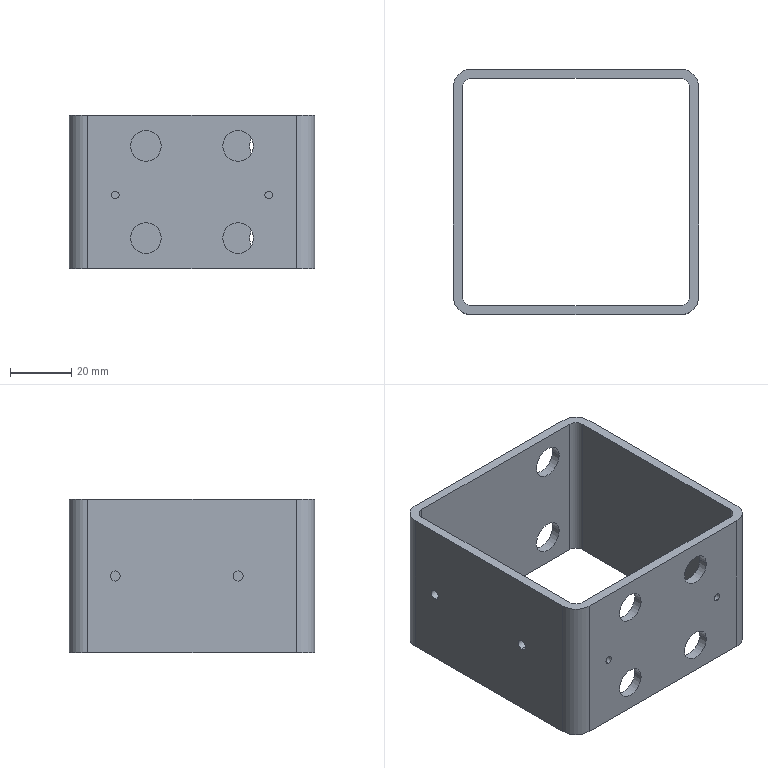Part | STEP file | X77-06302 | 1 solid | 38 faces | box 80 x 80 x 50 mm | volume 43498 mm3 | cylinder 28 | plane 10 | commonest cylinder face diameters 10 x8 2.5 x4 3.3 x4 6 x4 10.5 x4 12 x4
STEP:
#1=CARTESIAN_POINT('',(-19.91,-94.8,-15.));
#2=VERTEX_POINT('',#1);
#3=CARTESIAN_POINT('',(-29.91,-94.8,-15.));
#4=VERTEX_POINT('',#3);
#5=CARTESIAN_POINT('',(-24.91,-94.8,-15.));
#6=DIRECTION('',(0.,1.,0.));
#7=DIRECTION('',(0.,0.,-1.));
#8=AXIS2_PLACEMENT_3D('',#5,#6,#7);
#9=CIRCLE('',#8,5.);
#10=EDGE_CURVE('',#2,#4,#9,.T.);
#11=ORIENTED_EDGE('',*,*,#10,.T.);
#12=CARTESIAN_POINT('',(-29.91,-97.8,-15.));
#13=VERTEX_POINT('',#12);
#14=CARTESIAN_POINT('',(-29.91,-17.799,-15.));
#15=DIRECTION('',(0.,-1.,0.));
#16=VECTOR('',#15,1000.);
#17=LINE('',#14,#16);
#18=EDGE_CURVE('',#4,#13,#17,.T.);
#19=ORIENTED_EDGE('',*,*,#18,.T.);
#20=CARTESIAN_POINT('',(-19.91,-97.8,-15.));
#21=VERTEX_POINT('',#20);
#22=CARTESIAN_POINT('',(-24.91,-97.8,-15.));
#23=DIRECTION('',(0.,-1.,0.));
#24=DIRECTION('',(-1.,0.,0.));
#25=AXIS2_PLACEMENT_3D('',#22,#23,#24);
#26=CIRCLE('',#25,5.);
#27=EDGE_CURVE('',#13,#21,#26,.T.);
#28=ORIENTED_EDGE('',*,*,#27,.T.);
#29=CARTESIAN_POINT('',(-19.91,-17.799,-15.));
#30=DIRECTION('',(0.,-1.,0.));
#31=VECTOR('',#30,1000.);
#32=LINE('',#29,#31);
#33=EDGE_CURVE('',#2,#21,#32,.T.);
#34=ORIENTED_EDGE('',*,*,#33,.F.);
#35=EDGE_LOOP('',(#11,#19,#28,#34));
#36=FACE_OUTER_BOUND('',#35,.T.);
#37=CARTESIAN_POINT('',(-24.91,-17.799,-15.));
#38=DIRECTION('',(0.,-1.,0.));
#39=DIRECTION('',(1.,0.,0.));
#40=AXIS2_PLACEMENT_3D('',#37,#38,#39);
#41=CYLINDRICAL_SURFACE('',#40,5.);
#42=ADVANCED_FACE('',(#36),#41,.F.);
#43=CARTESIAN_POINT('',(10.09,-94.8,-15.));
#44=VERTEX_POINT('',#43);
#45=CARTESIAN_POINT('',(0.09,-94.8,-15.));
#46=VERTEX_POINT('',#45);
#47=CARTESIAN_POINT('',(5.09,-94.8,-15.));
#48=DIRECTION('',(0.,1.,0.));
#49=DIRECTION('',(0.,0.,-1.));
#50=AXIS2_PLACEMENT_3D('',#47,#48,#49);
#51=CIRCLE('',#50,5.);
#52=EDGE_CURVE('',#44,#46,#51,.T.);
#53=ORIENTED_EDGE('',*,*,#52,.T.);
#54=CARTESIAN_POINT('',(0.09,-97.8,-15.));
#55=VERTEX_POINT('',#54);
#56=CARTESIAN_POINT('',(0.09,-17.799,-15.));
#57=DIRECTION('',(0.,-1.,0.));
#58=VECTOR('',#57,1000.);
#59=LINE('',#56,#58);
#60=EDGE_CURVE('',#46,#55,#59,.T.);
#61=ORIENTED_EDGE('',*,*,#60,.T.);
#62=CARTESIAN_POINT('',(10.09,-97.8,-15.));
#63=VERTEX_POINT('',#62);
#64=CARTESIAN_POINT('',(5.09,-97.8,-15.));
#65=DIRECTION('',(0.,-1.,0.));
#66=DIRECTION('',(-1.,0.,0.));
#67=AXIS2_PLACEMENT_3D('',#64,#65,#66);
#68=CIRCLE('',#67,5.);
#69=EDGE_CURVE('',#55,#63,#68,.T.);
#70=ORIENTED_EDGE('',*,*,#69,.T.);
#71=CARTESIAN_POINT('',(10.09,-17.799,-15.));
#72=DIRECTION('',(0.,-1.,0.));
#73=VECTOR('',#72,1000.);
#74=LINE('',#71,#73);
#75=EDGE_CURVE('',#44,#63,#74,.T.);
#76=ORIENTED_EDGE('',*,*,#75,.F.);
#77=EDGE_LOOP('',(#53,#61,#70,#76));
#78=FACE_OUTER_BOUND('',#77,.T.);
#79=CARTESIAN_POINT('',(5.09,-17.799,-15.));
#80=DIRECTION('',(0.,-1.,0.));
#81=DIRECTION('',(1.,0.,0.));
#82=AXIS2_PLACEMENT_3D('',#79,#80,#81);
#83=CYLINDRICAL_SURFACE('',#82,5.);
#84=ADVANCED_FACE('',(#78),#83,.F.);
#85=CARTESIAN_POINT('',(-19.91,-94.8,15.));
#86=VERTEX_POINT('',#85);
#87=CARTESIAN_POINT('',(-29.91,-94.8,15.));
#88=VERTEX_POINT('',#87);
#89=CARTESIAN_POINT('',(-24.91,-94.8,15.));
#90=DIRECTION('',(0.,1.,0.));
#91=DIRECTION('',(0.,0.,-1.));
#92=AXIS2_PLACEMENT_3D('',#89,#90,#91);
#93=CIRCLE('',#92,5.);
#94=EDGE_CURVE('',#86,#88,#93,.T.);
#95=ORIENTED_EDGE('',*,*,#94,.T.);
#96=CARTESIAN_POINT('',(-29.91,-97.8,15.));
#97=VERTEX_POINT('',#96);
#98=CARTESIAN_POINT('',(-29.91,-17.799,15.));
#99=DIRECTION('',(0.,-1.,0.));
#100=VECTOR('',#99,1000.);
#101=LINE('',#98,#100);
#102=EDGE_CURVE('',#88,#97,#101,.T.);
#103=ORIENTED_EDGE('',*,*,#102,.T.);
#104=CARTESIAN_POINT('',(-19.91,-97.8,15.));
#105=VERTEX_POINT('',#104);
#106=CARTESIAN_POINT('',(-24.91,-97.8,15.));
#107=DIRECTION('',(0.,-1.,0.));
#108=DIRECTION('',(1.,0.,0.));
#109=AXIS2_PLACEMENT_3D('',#106,#107,#108);
#110=CIRCLE('',#109,5.);
#111=EDGE_CURVE('',#97,#105,#110,.T.);
#112=ORIENTED_EDGE('',*,*,#111,.T.);
#113=CARTESIAN_POINT('',(-19.91,-17.799,15.));
#114=DIRECTION('',(0.,-1.,0.));
#115=VECTOR('',#114,1000.);
#116=LINE('',#113,#115);
#117=EDGE_CURVE('',#86,#105,#116,.T.);
#118=ORIENTED_EDGE('',*,*,#117,.F.);
#119=EDGE_LOOP('',(#95,#103,#112,#118));
#120=FACE_OUTER_BOUND('',#119,.T.);
#121=CARTESIAN_POINT('',(-24.91,-17.799,15.));
#122=DIRECTION('',(0.,-1.,0.));
#123=DIRECTION('',(1.,0.,0.));
#124=AXIS2_PLACEMENT_3D('',#121,#122,#123);
#125=CYLINDRICAL_SURFACE('',#124,5.);
#126=ADVANCED_FACE('',(#120),#125,.F.);
#127=CARTESIAN_POINT('',(10.09,-94.8,15.));
#128=VERTEX_POINT('',#127);
#129=CARTESIAN_POINT('',(0.09,-94.8,15.));
#130=VERTEX_POINT('',#129);
#131=CARTESIAN_POINT('',(5.09,-94.8,15.));
#132=DIRECTION('',(0.,1.,0.));
#133=DIRECTION('',(0.,0.,-1.));
#134=AXIS2_PLACEMENT_3D('',#131,#132,#133);
#135=CIRCLE('',#134,5.);
#136=EDGE_CURVE('',#128,#130,#135,.T.);
#137=ORIENTED_EDGE('',*,*,#136,.T.);
#138=CARTESIAN_POINT('',(0.09,-97.8,15.));
#139=VERTEX_POINT('',#138);
#140=CARTESIAN_POINT('',(0.09,-17.799,15.));
#141=DIRECTION('',(0.,-1.,0.));
#142=VECTOR('',#141,1000.);
#143=LINE('',#140,#142);
#144=EDGE_CURVE('',#130,#139,#143,.T.);
#145=ORIENTED_EDGE('',*,*,#144,.T.);
#146=CARTESIAN_POINT('',(10.09,-97.8,15.));
#147=VERTEX_POINT('',#146);
#148=CARTESIAN_POINT('',(5.09,-97.8,15.));
#149=DIRECTION('',(0.,-1.,0.));
#150=DIRECTION('',(1.,0.,0.));
#151=AXIS2_PLACEMENT_3D('',#148,#149,#150);
#152=CIRCLE('',#151,5.);
#153=EDGE_CURVE('',#139,#147,#152,.T.);
#154=ORIENTED_EDGE('',*,*,#153,.T.);
#155=CARTESIAN_POINT('',(10.09,-17.799,15.));
#156=DIRECTION('',(0.,-1.,0.));
#157=VECTOR('',#156,1000.);
#158=LINE('',#155,#157);
#159=EDGE_CURVE('',#128,#147,#158,.T.);
#160=ORIENTED_EDGE('',*,*,#159,.F.);
#161=EDGE_LOOP('',(#137,#145,#154,#160));
#162=FACE_OUTER_BOUND('',#161,.T.);
#163=CARTESIAN_POINT('',(5.09,-17.799,15.));
#164=DIRECTION('',(0.,-1.,0.));
#165=DIRECTION('',(1.,0.,0.));
#166=AXIS2_PLACEMENT_3D('',#163,#164,#165);
#167=CYLINDRICAL_SURFACE('',#166,5.);
#168=ADVANCED_FACE('',(#162),#167,.F.);
#169=CARTESIAN_POINT('',(-34.91,-94.8,0.25));
#170=VERTEX_POINT('',#169);
#171=CARTESIAN_POINT('',(-34.91,-94.8,-2.25));
#172=VERTEX_POINT('',#171);
#173=CARTESIAN_POINT('',(-34.91,-94.8,-1.));
#174=DIRECTION('',(0.,-1.,0.));
#175=DIRECTION('',(0.,0.,-1.));
#176=AXIS2_PLACEMENT_3D('',#173,#174,#175);
#177=CIRCLE('',#176,1.25);
#178=EDGE_CURVE('',#170,#172,#177,.T.);
#179=ORIENTED_EDGE('',*,*,#178,.F.);
#180=CARTESIAN_POINT('',(-34.91,-97.8,0.25));
#181=VERTEX_POINT('',#180);
#182=CARTESIAN_POINT('',(-34.91,-97.8,0.25));
#183=DIRECTION('',(0.,-1.,0.));
#184=VECTOR('',#183,1000.);
#185=LINE('',#182,#184);
#186=EDGE_CURVE('',#170,#181,#185,.T.);
#187=ORIENTED_EDGE('',*,*,#186,.T.);
#188=CARTESIAN_POINT('',(-34.91,-97.8,-2.25));
#189=VERTEX_POINT('',#188);
#190=CARTESIAN_POINT('',(-34.91,-97.8,-1.));
#191=DIRECTION('',(0.,-1.,0.));
#192=DIRECTION('',(0.,0.,-1.));
#193=AXIS2_PLACEMENT_3D('',#190,#191,#192);
#194=CIRCLE('',#193,1.25);
#195=EDGE_CURVE('',#181,#189,#194,.T.);
#196=ORIENTED_EDGE('',*,*,#195,.T.);
#197=CARTESIAN_POINT('',(-34.91,-97.8,-2.25));
#198=DIRECTION('',(0.,-1.,0.));
#199=VECTOR('',#198,1000.);
#200=LINE('',#197,#199);
#201=EDGE_CURVE('',#172,#189,#200,.T.);
#202=ORIENTED_EDGE('',*,*,#201,.F.);
#203=EDGE_LOOP('',(#179,#187,#196,#202));
#204=FACE_OUTER_BOUND('',#203,.T.);
#205=CARTESIAN_POINT('',(-34.91,-97.8,-1.));
#206=DIRECTION('',(0.,-1.,0.));
#207=DIRECTION('',(0.,0.,-1.));
#208=AXIS2_PLACEMENT_3D('',#205,#206,#207);
#209=CYLINDRICAL_SURFACE('',#208,1.25);
#210=ADVANCED_FACE('',(#204),#209,.F.);
#211=CARTESIAN_POINT('',(15.09,-94.8,0.25));
#212=VERTEX_POINT('',#211);
#213=CARTESIAN_POINT('',(15.09,-94.8,-2.25));
#214=VERTEX_POINT('',#213);
#215=CARTESIAN_POINT('',(15.09,-94.8,-1.));
#216=DIRECTION('',(0.,-1.,0.));
#217=DIRECTION('',(0.,0.,-1.));
#218=AXIS2_PLACEMENT_3D('',#215,#216,#217);
#219=CIRCLE('',#218,1.25);
#220=EDGE_CURVE('',#212,#214,#219,.T.);
#221=ORIENTED_EDGE('',*,*,#220,.F.);
#222=CARTESIAN_POINT('',(15.09,-97.8,0.25));
#223=VERTEX_POINT('',#222);
#224=CARTESIAN_POINT('',(15.09,-97.8,0.25));
#225=DIRECTION('',(0.,-1.,0.));
#226=VECTOR('',#225,1000.);
#227=LINE('',#224,#226);
#228=EDGE_CURVE('',#212,#223,#227,.T.);
#229=ORIENTED_EDGE('',*,*,#228,.T.);
#230=CARTESIAN_POINT('',(15.09,-97.8,-2.25));
#231=VERTEX_POINT('',#230);
#232=CARTESIAN_POINT('',(15.09,-97.8,-1.));
#233=DIRECTION('',(0.,-1.,0.));
#234=DIRECTION('',(0.,0.,-1.));
#235=AXIS2_PLACEMENT_3D('',#232,#233,#234);
#236=CIRCLE('',#235,1.25);
#237=EDGE_CURVE('',#223,#231,#236,.T.);
#238=ORIENTED_EDGE('',*,*,#237,.T.);
#239=CARTESIAN_POINT('',(15.09,-97.8,-2.25));
#240=DIRECTION('',(0.,-1.,0.));
#241=VECTOR('',#240,1000.);
#242=LINE('',#239,#241);
#243=EDGE_CURVE('',#214,#231,#242,.T.);
#244=ORIENTED_EDGE('',*,*,#243,.F.);
#245=EDGE_LOOP('',(#221,#229,#238,#244));
#246=FACE_OUTER_BOUND('',#245,.T.);
#247=CARTESIAN_POINT('',(15.09,-97.8,-1.));
#248=DIRECTION('',(0.,-1.,0.));
#249=DIRECTION('',(0.,0.,-1.));
#250=AXIS2_PLACEMENT_3D('',#247,#248,#249);
#251=CYLINDRICAL_SURFACE('',#250,1.25);
#252=ADVANCED_FACE('',(#246),#251,.F.);
#253=CARTESIAN_POINT('',(8.84,-17.8,-15.));
#254=VERTEX_POINT('',#253);
#255=CARTESIAN_POINT('',(19.34,-17.8,-15.));
#256=VERTEX_POINT('',#255);
#257=CARTESIAN_POINT('',(14.09,-17.8,-15.));
#258=DIRECTION('',(0.,-1.,0.));
#259=DIRECTION('',(1.,0.,0.));
#260=AXIS2_PLACEMENT_3D('',#257,#258,#259);
#261=CIRCLE('',#260,5.25);
#262=EDGE_CURVE('',#254,#256,#261,.T.);
#263=ORIENTED_EDGE('',*,*,#262,.F.);
#264=CARTESIAN_POINT('',(8.84,-20.8,-15.));
#265=VERTEX_POINT('',#264);
#266=CARTESIAN_POINT('',(8.84,-17.8,-15.));
#267=DIRECTION('',(0.,-1.,0.));
#268=VECTOR('',#267,1000.);
#269=LINE('',#266,#268);
#270=EDGE_CURVE('',#254,#265,#269,.T.);
#271=ORIENTED_EDGE('',*,*,#270,.T.);
#272=CARTESIAN_POINT('',(19.34,-20.8,-15.));
#273=VERTEX_POINT('',#272);
#274=CARTESIAN_POINT('',(14.09,-20.8,-15.));
#275=DIRECTION('',(0.,-1.,0.));
#276=DIRECTION('',(1.,0.,0.));
#277=AXIS2_PLACEMENT_3D('',#274,#275,#276);
#278=CIRCLE('',#277,5.25);
#279=EDGE_CURVE('',#265,#273,#278,.T.);
#280=ORIENTED_EDGE('',*,*,#279,.T.);
#281=CARTESIAN_POINT('',(19.34,-17.8,-15.));
#282=DIRECTION('',(0.,-1.,0.));
#283=VECTOR('',#282,1000.);
#284=LINE('',#281,#283);
#285=EDGE_CURVE('',#256,#273,#284,.T.);
#286=ORIENTED_EDGE('',*,*,#285,.F.);
#287=EDGE_LOOP('',(#263,#271,#280,#286));
#288=FACE_OUTER_BOUND('',#287,.T.);
#289=CARTESIAN_POINT('',(14.09,-17.8,-15.));
#290=DIRECTION('',(0.,-1.,0.));
#291=DIRECTION('',(1.,0.,0.));
#292=AXIS2_PLACEMENT_3D('',#289,#290,#291);
#293=CYLINDRICAL_SURFACE('',#292,5.25);
#294=ADVANCED_FACE('',(#288),#293,.F.);
#295=CARTESIAN_POINT('',(8.84,-17.8,15.));
#296=VERTEX_POINT('',#295);
#297=CARTESIAN_POINT('',(19.34,-17.8,15.));
#298=VERTEX_POINT('',#297);
#299=CARTESIAN_POINT('',(14.09,-17.8,15.));
#300=DIRECTION('',(0.,-1.,0.));
#301=DIRECTION('',(1.,0.,0.));
#302=AXIS2_PLACEMENT_3D('',#299,#300,#301);
#303=CIRCLE('',#302,5.25);
#304=EDGE_CURVE('',#296,#298,#303,.T.);
#305=ORIENTED_EDGE('',*,*,#304,.F.);
#306=CARTESIAN_POINT('',(8.84,-20.8,15.));
#307=VERTEX_POINT('',#306);
#308=CARTESIAN_POINT('',(8.84,-17.8,15.));
#309=DIRECTION('',(0.,-1.,0.));
#310=VECTOR('',#309,1000.);
#311=LINE('',#308,#310);
#312=EDGE_CURVE('',#296,#307,#311,.T.);
#313=ORIENTED_EDGE('',*,*,#312,.T.);
#314=CARTESIAN_POINT('',(19.34,-20.8,15.));
#315=VERTEX_POINT('',#314);
#316=CARTESIAN_POINT('',(14.09,-20.8,15.));
#317=DIRECTION('',(0.,-1.,0.));
#318=DIRECTION('',(1.,0.,0.));
#319=AXIS2_PLACEMENT_3D('',#316,#317,#318);
#320=CIRCLE('',#319,5.25);
#321=EDGE_CURVE('',#307,#315,#320,.T.);
#322=ORIENTED_EDGE('',*,*,#321,.T.);
#323=CARTESIAN_POINT('',(19.34,-17.8,15.));
#324=DIRECTION('',(0.,-1.,0.));
#325=VECTOR('',#324,1000.);
#326=LINE('',#323,#325);
#327=EDGE_CURVE('',#298,#315,#326,.T.);
#328=ORIENTED_EDGE('',*,*,#327,.F.);
#329=EDGE_LOOP('',(#305,#313,#322,#328));
#330=FACE_OUTER_BOUND('',#329,.T.);
#331=CARTESIAN_POINT('',(14.09,-17.8,15.));
#332=DIRECTION('',(0.,-1.,0.));
#333=DIRECTION('',(1.,0.,0.));
#334=AXIS2_PLACEMENT_3D('',#331,#332,#333);
#335=CYLINDRICAL_SURFACE('',#334,5.25);
#336=ADVANCED_FACE('',(#330),#335,.F.);
#337=CARTESIAN_POINT('',(-46.91,-72.8,-1.65));
#338=VERTEX_POINT('',#337);
#339=CARTESIAN_POINT('',(-46.91,-72.8,1.65));
#340=VERTEX_POINT('',#339);
#341=CARTESIAN_POINT('',(-46.91,-72.8,0.));
#342=DIRECTION('',(-1.,0.,0.));
#343=DIRECTION('',(0.,-1.,0.));
#344=AXIS2_PLACEMENT_3D('',#341,#342,#343);
#345=CIRCLE('',#344,1.65);
#346=EDGE_CURVE('',#338,#340,#345,.T.);
#347=ORIENTED_EDGE('',*,*,#346,.F.);
#348=CARTESIAN_POINT('',(-49.91,-72.8,-1.65));
#349=VERTEX_POINT('',#348);
#350=CARTESIAN_POINT('',(-49.91,-72.8,-1.65));
#351=DIRECTION('',(-1.,0.,0.));
#352=VECTOR('',#351,1000.);
#353=LINE('',#350,#352);
#354=EDGE_CURVE('',#338,#349,#353,.T.);
#355=ORIENTED_EDGE('',*,*,#354,.T.);
#356=CARTESIAN_POINT('',(-49.91,-72.8,1.65));
#357=VERTEX_POINT('',#356);
#358=CARTESIAN_POINT('',(-49.91,-72.8,0.));
#359=DIRECTION('',(-1.,0.,0.));
#360=DIRECTION('',(0.,0.,1.));
#361=AXIS2_PLACEMENT_3D('',#358,#359,#360);
#362=CIRCLE('',#361,1.65);
#363=EDGE_CURVE('',#349,#357,#362,.T.);
#364=ORIENTED_EDGE('',*,*,#363,.T.);
#365=CARTESIAN_POINT('',(-49.91,-72.8,1.65));
#366=DIRECTION('',(-1.,0.,0.));
#367=VECTOR('',#366,1000.);
#368=LINE('',#365,#367);
#369=EDGE_CURVE('',#340,#357,#368,.T.);
#370=ORIENTED_EDGE('',*,*,#369,.F.);
#371=EDGE_LOOP('',(#347,#355,#364,#370));
#372=FACE_OUTER_BOUND('',#371,.T.);
#373=CARTESIAN_POINT('',(-49.91,-72.8,0.));
#374=DIRECTION('',(-1.,0.,0.));
#375=DIRECTION('',(0.,0.,1.));
#376=AXIS2_PLACEMENT_3D('',#373,#374,#375);
#377=CYLINDRICAL_SURFACE('',#376,1.65);
#378=ADVANCED_FACE('',(#372),#377,.F.);
#379=CARTESIAN_POINT('',(-46.91,-32.8,-1.65));
#380=VERTEX_POINT('',#379);
#381=CARTESIAN_POINT('',(-46.91,-32.8,1.65));
#382=VERTEX_POINT('',#381);
#383=CARTESIAN_POINT('',(-46.91,-32.8,0.));
#384=DIRECTION('',(-1.,0.,0.));
#385=DIRECTION('',(0.,-1.,0.));
#386=AXIS2_PLACEMENT_3D('',#383,#384,#385);
#387=CIRCLE('',#386,1.65);
#388=EDGE_CURVE('',#380,#382,#387,.T.);
#389=ORIENTED_EDGE('',*,*,#388,.F.);
#390=CARTESIAN_POINT('',(-49.91,-32.8,-1.65));
#391=VERTEX_POINT('',#390);
#392=CARTESIAN_POINT('',(-49.91,-32.8,-1.65));
#393=DIRECTION('',(-1.,0.,0.));
#394=VECTOR('',#393,1000.);
#395=LINE('',#392,#394);
#396=EDGE_CURVE('',#380,#391,#395,.T.);
#397=ORIENTED_EDGE('',*,*,#396,.T.);
#398=CARTESIAN_POINT('',(-49.91,-32.8,1.65));
#399=VERTEX_POINT('',#398);
#400=CARTESIAN_POINT('',(-49.91,-32.8,0.));
#401=DIRECTION('',(-1.,0.,0.));
#402=DIRECTION('',(0.,0.,1.));
#403=AXIS2_PLACEMENT_3D('',#400,#401,#402);
#404=CIRCLE('',#403,1.65);
#405=EDGE_CURVE('',#391,#399,#404,.T.);
#406=ORIENTED_EDGE('',*,*,#405,.T.);
#407=CARTESIAN_POINT('',(-49.91,-32.8,1.65));
#408=DIRECTION('',(-1.,0.,0.));
#409=VECTOR('',#408,1000.);
#410=LINE('',#407,#409);
#411=EDGE_CURVE('',#382,#399,#410,.T.);
#412=ORIENTED_EDGE('',*,*,#411,.F.);
#413=EDGE_LOOP('',(#389,#397,#406,#412));
#414=FACE_OUTER_BOUND('',#413,.T.);
#415=CARTESIAN_POINT('',(-49.91,-32.8,0.));
#416=DIRECTION('',(-1.,0.,0.));
#417=DIRECTION('',(0.,0.,1.));
#418=AXIS2_PLACEMENT_3D('',#415,#416,#417);
#419=CYLINDRICAL_SURFACE('',#418,1.65);
#420=ADVANCED_FACE('',(#414),#419,.F.);
#421=CARTESIAN_POINT('',(-49.91,-23.8,-25.));
#422=VERTEX_POINT('',#421);
#423=CARTESIAN_POINT('',(-49.91,-23.8,25.));
#424=VERTEX_POINT('',#423);
#425=CARTESIAN_POINT('',(-49.91,-23.8,-25.));
#426=DIRECTION('',(0.,0.,1.));
#427=VECTOR('',#426,1000.);
#428=LINE('',#425,#427);
#429=EDGE_CURVE('',#422,#424,#428,.T.);
#430=ORIENTED_EDGE('',*,*,#429,.T.);
#431=CARTESIAN_POINT('',(-43.91,-17.8,25.));
#432=VERTEX_POINT('',#431);
#433=CARTESIAN_POINT('',(-43.91,-23.8,25.));
#434=DIRECTION('',(0.,0.,1.));
#435=DIRECTION('',(-1.,0.,0.));
#436=AXIS2_PLACEMENT_3D('',#433,#434,#435);
#437=CIRCLE('',#436,6.);
#438=EDGE_CURVE('',#432,#424,#437,.T.);
#439=ORIENTED_EDGE('',*,*,#438,.F.);
#440=CARTESIAN_POINT('',(-43.91,-17.8,-25.));
#441=VERTEX_POINT('',#440);
#442=CARTESIAN_POINT('',(-43.91,-17.8,-25.));
#443=DIRECTION('',(0.,0.,1.));
#444=VECTOR('',#443,1000.);
#445=LINE('',#442,#444);
#446=EDGE_CURVE('',#441,#432,#445,.T.);
#447=ORIENTED_EDGE('',*,*,#446,.F.);
#448=CARTESIAN_POINT('',(-43.91,-23.8,-25.));
#449=DIRECTION('',(0.,0.,1.));
#450=DIRECTION('',(-1.,0.,0.));
#451=AXIS2_PLACEMENT_3D('',#448,#449,#450);
#452=CIRCLE('',#451,6.);
#453=EDGE_CURVE('',#441,#422,#452,.T.);
#454=ORIENTED_EDGE('',*,*,#453,.T.);
#455=EDGE_LOOP('',(#430,#439,#447,#454));
#456=FACE_OUTER_BOUND('',#455,.T.);
#457=CARTESIAN_POINT('',(-43.91,-23.8,-25.));
#458=DIRECTION('',(0.,0.,1.));
#459=DIRECTION('',(1.,0.,0.));
#460=AXIS2_PLACEMENT_3D('',#457,#458,#459);
#461=CYLINDRICAL_SURFACE('',#460,6.);
#462=ADVANCED_FACE('',(#456),#461,.T.);
#463=CARTESIAN_POINT('',(14.09,-17.8,-15.));
#464=DIRECTION('',(0.,-1.,0.));
#465=DIRECTION('',(1.,0.,0.));
#466=AXIS2_PLACEMENT_3D('',#463,#464,#465);
#467=CIRCLE('',#466,5.25);
#468=EDGE_CURVE('',#256,#254,#467,.T.);
#469=ORIENTED_EDGE('',*,*,#468,.T.);
#470=ORIENTED_EDGE('',*,*,#262,.T.);
#471=EDGE_LOOP('',(#469,#470));
#472=FACE_BOUND('',#471,.T.);
#473=CARTESIAN_POINT('',(14.09,-17.8,15.));
#474=DIRECTION('',(0.,-1.,0.));
#475=DIRECTION('',(1.,0.,0.));
#476=AXIS2_PLACEMENT_3D('',#473,#474,#475);
#477=CIRCLE('',#476,5.25);
#478=EDGE_CURVE('',#298,#296,#477,.T.);
#479=ORIENTED_EDGE('',*,*,#478,.T.);
#480=ORIENTED_EDGE('',*,*,#304,.T.);
#481=EDGE_LOOP('',(#479,#480));
#482=FACE_BOUND('',#481,.T.);
#483=ORIENTED_EDGE('',*,*,#446,.T.);
#484=CARTESIAN_POINT('',(24.09,-17.8,25.));
#485=VERTEX_POINT('',#484);
#486=CARTESIAN_POINT('',(24.09,-17.8,25.));
#487=DIRECTION('',(-1.,0.,0.));
#488=VECTOR('',#487,1000.);
#489=LINE('',#486,#488);
#490=EDGE_CURVE('',#485,#432,#489,.T.);
#491=ORIENTED_EDGE('',*,*,#490,.F.);
#492=CARTESIAN_POINT('',(24.09,-17.8,-25.));
#493=VERTEX_POINT('',#492);
#494=CARTESIAN_POINT('',(24.09,-17.8,-25.));
#495=DIRECTION('',(0.,0.,1.));
#496=VECTOR('',#495,1000.);
#497=LINE('',#494,#496);
#498=EDGE_CURVE('',#493,#485,#497,.T.);
#499=ORIENTED_EDGE('',*,*,#498,.F.);
#500=CARTESIAN_POINT('',(24.09,-17.8,-25.));
#501=DIRECTION('',(-1.,0.,0.));
#502=VECTOR('',#501,1000.);
#503=LINE('',#500,#502);
#504=EDGE_CURVE('',#493,#441,#503,.T.);
#505=ORIENTED_EDGE('',*,*,#504,.T.);
#506=EDGE_LOOP('',(#483,#491,#499,#505));
#507=FACE_OUTER_BOUND('',#506,.T.);
#508=CARTESIAN_POINT('',(24.09,-17.8,-25.));
#509=DIRECTION('',(0.,1.,0.));
#510=DIRECTION('',(-1.,0.,0.));
#511=AXIS2_PLACEMENT_3D('',#508,#509,#510);
#512=PLANE('',#511);
#513=ADVANCED_FACE('',(#472,#482,#507),#512,.T.);
#514=ORIENTED_EDGE('',*,*,#498,.T.);
#515=CARTESIAN_POINT('',(30.09,-23.8,25.));
#516=VERTEX_POINT('',#515);
#517=CARTESIAN_POINT('',(24.09,-23.8,25.));
#518=DIRECTION('',(0.,0.,1.));
#519=DIRECTION('',(1.,0.,0.));
#520=AXIS2_PLACEMENT_3D('',#517,#518,#519);
#521=CIRCLE('',#520,6.);
#522=EDGE_CURVE('',#516,#485,#521,.T.);
#523=ORIENTED_EDGE('',*,*,#522,.F.);
#524=CARTESIAN_POINT('',(30.09,-23.8,-25.));
#525=VERTEX_POINT('',#524);
#526=CARTESIAN_POINT('',(30.09,-23.8,-25.));
#527=DIRECTION('',(0.,0.,1.));
#528=VECTOR('',#527,1000.);
#529=LINE('',#526,#528);
#530=EDGE_CURVE('',#525,#516,#529,.T.);
#531=ORIENTED_EDGE('',*,*,#530,.F.);
#532=CARTESIAN_POINT('',(24.09,-23.8,-25.));
#533=DIRECTION('',(0.,0.,1.));
#534=DIRECTION('',(1.,0.,0.));
#535=AXIS2_PLACEMENT_3D('',#532,#533,#534);
#536=CIRCLE('',#535,6.);
#537=EDGE_CURVE('',#525,#493,#536,.T.);
#538=ORIENTED_EDGE('',*,*,#537,.T.);
#539=EDGE_LOOP('',(#514,#523,#531,#538));
#540=FACE_OUTER_BOUND('',#539,.T.);
#541=CARTESIAN_POINT('',(24.09,-23.8,-25.));
#542=DIRECTION('',(0.,0.,1.));
#543=DIRECTION('',(1.,0.,0.));
#544=AXIS2_PLACEMENT_3D('',#541,#542,#543);
#545=CYLINDRICAL_SURFACE('',#544,6.);
#546=ADVANCED_FACE('',(#540),#545,.T.);
#547=ORIENTED_EDGE('',*,*,#530,.T.);
#548=CARTESIAN_POINT('',(30.09,-91.8,25.));
#549=VERTEX_POINT('',#548);
#550=CARTESIAN_POINT('',(30.09,-23.8,25.));
#551=DIRECTION('',(0.,1.,0.));
#552=VECTOR('',#551,1000.);
#553=LINE('',#550,#552);
#554=EDGE_CURVE('',#549,#516,#553,.T.);
#555=ORIENTED_EDGE('',*,*,#554,.F.);
#556=CARTESIAN_POINT('',(30.09,-91.8,-25.));
#557=VERTEX_POINT('',#556);
#558=CARTESIAN_POINT('',(30.09,-91.8,-25.));
#559=DIRECTION('',(0.,0.,1.));
#560=VECTOR('',#559,1000.);
#561=LINE('',#558,#560);
#562=EDGE_CURVE('',#557,#549,#561,.T.);
#563=ORIENTED_EDGE('',*,*,#562,.F.);
#564=CARTESIAN_POINT('',(30.09,-23.8,-25.));
#565=DIRECTION('',(0.,1.,0.));
#566=VECTOR('',#565,1000.);
#567=LINE('',#564,#566);
#568=EDGE_CURVE('',#557,#525,#567,.T.);
#569=ORIENTED_EDGE('',*,*,#568,.T.);
#570=EDGE_LOOP('',(#547,#555,#563,#569));
#571=FACE_OUTER_BOUND('',#570,.T.);
#572=CARTESIAN_POINT('',(30.09,-23.8,-25.));
#573=DIRECTION('',(1.,0.,0.));
#574=DIRECTION('',(0.,1.,0.));
#575=AXIS2_PLACEMENT_3D('',#572,#573,#574);
#576=PLANE('',#575);
#577=ADVANCED_FACE('',(#571),#576,.T.);
#578=ORIENTED_EDGE('',*,*,#562,.T.);
#579=CARTESIAN_POINT('',(24.09,-97.8,25.));
#580=VERTEX_POINT('',#579);
#581=CARTESIAN_POINT('',(24.09,-91.8,25.));
#582=DIRECTION('',(0.,0.,1.));
#583=DIRECTION('',(-1.,0.,0.));
#584=AXIS2_PLACEMENT_3D('',#581,#582,#583);
#585=CIRCLE('',#584,6.);
#586=EDGE_CURVE('',#580,#549,#585,.T.);
#587=ORIENTED_EDGE('',*,*,#586,.F.);
#588=CARTESIAN_POINT('',(24.09,-97.8,-25.));
#589=VERTEX_POINT('',#588);
#590=CARTESIAN_POINT('',(24.09,-97.8,-25.));
#591=DIRECTION('',(0.,0.,1.));
#592=VECTOR('',#591,1000.);
#593=LINE('',#590,#592);
#594=EDGE_CURVE('',#589,#580,#593,.T.);
#595=ORIENTED_EDGE('',*,*,#594,.F.);
#596=CARTESIAN_POINT('',(24.09,-91.8,-25.));
#597=DIRECTION('',(0.,0.,1.));
#598=DIRECTION('',(-1.,0.,0.));
#599=AXIS2_PLACEMENT_3D('',#596,#597,#598);
#600=CIRCLE('',#599,6.);
#601=EDGE_CURVE('',#589,#557,#600,.T.);
#602=ORIENTED_EDGE('',*,*,#601,.T.);
#603=EDGE_LOOP('',(#578,#587,#595,#602));
#604=FACE_OUTER_BOUND('',#603,.T.);
#605=CARTESIAN_POINT('',(24.09,-91.8,-25.));
#606=DIRECTION('',(0.,0.,1.));
#607=DIRECTION('',(1.,0.,0.));
#608=AXIS2_PLACEMENT_3D('',#605,#606,#607);
#609=CYLINDRICAL_SURFACE('',#608,6.);
#610=ADVANCED_FACE('',(#604),#609,.T.);
#611=CARTESIAN_POINT('',(-24.91,-97.8,-15.));
#612=DIRECTION('',(0.,-1.,0.));
#613=DIRECTION('',(-1.,0.,0.));
#614=AXIS2_PLACEMENT_3D('',#611,#612,#613);
#615=CIRCLE('',#614,5.);
#616=EDGE_CURVE('',#21,#13,#615,.T.);
#617=ORIENTED_EDGE('',*,*,#616,.F.);
#618=ORIENTED_EDGE('',*,*,#27,.F.);
#619=EDGE_LOOP('',(#617,#618));
#620=FACE_BOUND('',#619,.T.);
#621=CARTESIAN_POINT('',(5.09,-97.8,-15.));
#622=DIRECTION('',(0.,-1.,0.));
#623=DIRECTION('',(-1.,0.,0.));
#624=AXIS2_PLACEMENT_3D('',#621,#622,#623);
#625=CIRCLE('',#624,5.);
#626=EDGE_CURVE('',#63,#55,#625,.T.);
#627=ORIENTED_EDGE('',*,*,#626,.F.);
#628=ORIENTED_EDGE('',*,*,#69,.F.);
#629=EDGE_LOOP('',(#627,#628));
#630=FACE_BOUND('',#629,.T.);
#631=CARTESIAN_POINT('',(-24.91,-97.8,15.));
#632=DIRECTION('',(0.,-1.,0.));
#633=DIRECTION('',(1.,0.,0.));
#634=AXIS2_PLACEMENT_3D('',#631,#632,#633);
#635=CIRCLE('',#634,5.);
#636=EDGE_CURVE('',#105,#97,#635,.T.);
#637=ORIENTED_EDGE('',*,*,#636,.F.);
#638=ORIENTED_EDGE('',*,*,#111,.F.);
#639=EDGE_LOOP('',(#637,#638));
#640=FACE_BOUND('',#639,.T.);
#641=CARTESIAN_POINT('',(5.09,-97.8,15.));
#642=DIRECTION('',(0.,-1.,0.));
#643=DIRECTION('',(1.,0.,0.));
#644=AXIS2_PLACEMENT_3D('',#641,#642,#643);
#645=CIRCLE('',#644,5.);
#646=EDGE_CURVE('',#147,#139,#645,.T.);
#647=ORIENTED_EDGE('',*,*,#646,.F.);
#648=ORIENTED_EDGE('',*,*,#153,.F.);
#649=EDGE_LOOP('',(#647,#648));
#650=FACE_BOUND('',#649,.T.);
#651=CARTESIAN_POINT('',(-34.91,-97.8,-1.));
#652=DIRECTION('',(0.,-1.,0.));
#653=DIRECTION('',(0.,0.,-1.));
#654=AXIS2_PLACEMENT_3D('',#651,#652,#653);
#655=CIRCLE('',#654,1.25);
#656=EDGE_CURVE('',#189,#181,#655,.T.);
#657=ORIENTED_EDGE('',*,*,#656,.F.);
#658=ORIENTED_EDGE('',*,*,#195,.F.);
#659=EDGE_LOOP('',(#657,#658));
#660=FACE_BOUND('',#659,.T.);
#661=CARTESIAN_POINT('',(15.09,-97.8,-1.));
#662=DIRECTION('',(0.,-1.,0.));
#663=DIRECTION('',(0.,0.,-1.));
#664=AXIS2_PLACEMENT_3D('',#661,#662,#663);
#665=CIRCLE('',#664,1.25);
#666=EDGE_CURVE('',#231,#223,#665,.T.);
#667=ORIENTED_EDGE('',*,*,#666,.F.);
#668=ORIENTED_EDGE('',*,*,#237,.F.);
#669=EDGE_LOOP('',(#667,#668));
#670=FACE_BOUND('',#669,.T.);
#671=ORIENTED_EDGE('',*,*,#594,.T.);
#672=CARTESIAN_POINT('',(-43.91,-97.8,25.));
#673=VERTEX_POINT('',#672);
#674=CARTESIAN_POINT('',(-43.91,-97.8,25.));
#675=DIRECTION('',(1.,0.,0.));
#676=VECTOR('',#675,1000.);
#677=LINE('',#674,#676);
#678=EDGE_CURVE('',#673,#580,#677,.T.);
#679=ORIENTED_EDGE('',*,*,#678,.F.);
#680=CARTESIAN_POINT('',(-43.91,-97.8,-25.));
#681=VERTEX_POINT('',#680);
#682=CARTESIAN_POINT('',(-43.91,-97.8,-25.));
#683=DIRECTION('',(0.,0.,1.));
#684=VECTOR('',#683,1000.);
#685=LINE('',#682,#684);
#686=EDGE_CURVE('',#681,#673,#685,.T.);
#687=ORIENTED_EDGE('',*,*,#686,.F.);
#688=CARTESIAN_POINT('',(-43.91,-97.8,-25.));
#689=DIRECTION('',(1.,0.,0.));
#690=VECTOR('',#689,1000.);
#691=LINE('',#688,#690);
#692=EDGE_CURVE('',#681,#589,#691,.T.);
#693=ORIENTED_EDGE('',*,*,#692,.T.);
#694=EDGE_LOOP('',(#671,#679,#687,#693));
#695=FACE_OUTER_BOUND('',#694,.T.);
#696=CARTESIAN_POINT('',(-43.91,-97.8,-25.));
#697=DIRECTION('',(0.,-1.,0.));
#698=DIRECTION('',(1.,0.,0.));
#699=AXIS2_PLACEMENT_3D('',#696,#697,#698);
#700=PLANE('',#699);
#701=ADVANCED_FACE('',(#620,#630,#640,#650,#660,#670,#695),#700,.T.);
#702=ORIENTED_EDGE('',*,*,#686,.T.);
#703=CARTESIAN_POINT('',(-49.91,-91.8,25.));
#704=VERTEX_POINT('',#703);
#705=CARTESIAN_POINT('',(-43.91,-91.8,25.));
#706=DIRECTION('',(0.,0.,1.));
#707=DIRECTION('',(-1.,0.,0.));
#708=AXIS2_PLACEMENT_3D('',#705,#706,#707);
#709=CIRCLE('',#708,6.);
#710=EDGE_CURVE('',#704,#673,#709,.T.);
#711=ORIENTED_EDGE('',*,*,#710,.F.);
#712=CARTESIAN_POINT('',(-49.91,-91.8,-25.));
#713=VERTEX_POINT('',#712);
#714=CARTESIAN_POINT('',(-49.91,-91.8,-25.));
#715=DIRECTION('',(0.,0.,1.));
#716=VECTOR('',#715,1000.);
#717=LINE('',#714,#716);
#718=EDGE_CURVE('',#713,#704,#717,.T.);
#719=ORIENTED_EDGE('',*,*,#718,.F.);
#720=CARTESIAN_POINT('',(-43.91,-91.8,-25.));
#721=DIRECTION('',(0.,0.,1.));
#722=DIRECTION('',(-1.,0.,0.));
#723=AXIS2_PLACEMENT_3D('',#720,#721,#722);
#724=CIRCLE('',#723,6.);
#725=EDGE_CURVE('',#713,#681,#724,.T.);
#726=ORIENTED_EDGE('',*,*,#725,.T.);
#727=EDGE_LOOP('',(#702,#711,#719,#726));
#728=FACE_OUTER_BOUND('',#727,.T.);
#729=CARTESIAN_POINT('',(-43.91,-91.8,-25.));
#730=DIRECTION('',(0.,0.,1.));
#731=DIRECTION('',(1.,0.,0.));
#732=AXIS2_PLACEMENT_3D('',#729,#730,#731);
#733=CYLINDRICAL_SURFACE('',#732,6.);
#734=ADVANCED_FACE('',(#728),#733,.T.);
#735=CARTESIAN_POINT('',(-49.91,-72.8,0.));
#736=DIRECTION('',(-1.,0.,0.));
#737=DIRECTION('',(0.,0.,1.));
#738=AXIS2_PLACEMENT_3D('',#735,#736,#737);
#739=CIRCLE('',#738,1.65);
#740=EDGE_CURVE('',#357,#349,#739,.T.);
#741=ORIENTED_EDGE('',*,*,#740,.F.);
#742=ORIENTED_EDGE('',*,*,#363,.F.);
#743=EDGE_LOOP('',(#741,#742));
#744=FACE_BOUND('',#743,.T.);
#745=CARTESIAN_POINT('',(-49.91,-32.8,0.));
#746=DIRECTION('',(-1.,0.,0.));
#747=DIRECTION('',(0.,0.,1.));
#748=AXIS2_PLACEMENT_3D('',#745,#746,#747);
#749=CIRCLE('',#748,1.65);
#750=EDGE_CURVE('',#399,#391,#749,.T.);
#751=ORIENTED_EDGE('',*,*,#750,.F.);
#752=ORIENTED_EDGE('',*,*,#405,.F.);
#753=EDGE_LOOP('',(#751,#752));
#754=FACE_BOUND('',#753,.T.);
#755=ORIENTED_EDGE('',*,*,#718,.T.);
#756=CARTESIAN_POINT('',(-49.91,-23.8,25.));
#757=DIRECTION('',(0.,-1.,0.));
#758=VECTOR('',#757,1000.);
#759=LINE('',#756,#758);
#760=EDGE_CURVE('',#424,#704,#759,.T.);
#761=ORIENTED_EDGE('',*,*,#760,.F.);
#762=ORIENTED_EDGE('',*,*,#429,.F.);
#763=CARTESIAN_POINT('',(-49.91,-23.8,-25.));
#764=DIRECTION('',(0.,-1.,0.));
#765=VECTOR('',#764,1000.);
#766=LINE('',#763,#765);
#767=EDGE_CURVE('',#422,#713,#766,.T.);
#768=ORIENTED_EDGE('',*,*,#767,.T.);
#769=EDGE_LOOP('',(#755,#761,#762,#768));
#770=FACE_OUTER_BOUND('',#769,.T.);
#771=CARTESIAN_POINT('',(-49.91,-23.8,-25.));
#772=DIRECTION('',(-1.,0.,0.));
#773=DIRECTION('',(0.,-1.,0.));
#774=AXIS2_PLACEMENT_3D('',#771,#772,#773);
#775=PLANE('',#774);
#776=ADVANCED_FACE('',(#744,#754,#770),#775,.T.);
#777=CARTESIAN_POINT('',(27.09,-23.8,-25.));
#778=VERTEX_POINT('',#777);
#779=CARTESIAN_POINT('',(24.09,-20.8,-25.));
#780=VERTEX_POINT('',#779);
#781=CARTESIAN_POINT('',(24.09,-23.8,-25.));
#782=DIRECTION('',(0.,0.,1.));
#783=DIRECTION('',(1.,0.,0.));
#784=AXIS2_PLACEMENT_3D('',#781,#782,#783);
#785=CIRCLE('',#784,3.);
#786=EDGE_CURVE('',#778,#780,#785,.T.);
#787=ORIENTED_EDGE('',*,*,#786,.T.);
#788=CARTESIAN_POINT('',(-43.91,-20.8,-25.));
#789=VERTEX_POINT('',#788);
#790=CARTESIAN_POINT('',(24.09,-20.8,-25.));
#791=DIRECTION('',(-1.,0.,0.));
#792=VECTOR('',#791,1000.);
#793=LINE('',#790,#792);
#794=EDGE_CURVE('',#780,#789,#793,.T.);
#795=ORIENTED_EDGE('',*,*,#794,.T.);
#796=CARTESIAN_POINT('',(-46.91,-23.8,-25.));
#797=VERTEX_POINT('',#796);
#798=CARTESIAN_POINT('',(-43.91,-23.8,-25.));
#799=DIRECTION('',(0.,0.,1.));
#800=DIRECTION('',(-1.,0.,0.));
#801=AXIS2_PLACEMENT_3D('',#798,#799,#800);
#802=CIRCLE('',#801,3.);
#803=EDGE_CURVE('',#789,#797,#802,.T.);
#804=ORIENTED_EDGE('',*,*,#803,.T.);
#805=CARTESIAN_POINT('',(-46.91,-91.8,-25.));
#806=VERTEX_POINT('',#805);
#807=CARTESIAN_POINT('',(-46.91,-23.8,-25.));
#808=DIRECTION('',(0.,-1.,0.));
#809=VECTOR('',#808,1000.);
#810=LINE('',#807,#809);
#811=EDGE_CURVE('',#797,#806,#810,.T.);
#812=ORIENTED_EDGE('',*,*,#811,.T.);
#813=CARTESIAN_POINT('',(-43.91,-94.8,-25.));
#814=VERTEX_POINT('',#813);
#815=CARTESIAN_POINT('',(-43.91,-91.8,-25.));
#816=DIRECTION('',(0.,0.,1.));
#817=DIRECTION('',(-1.,0.,0.));
#818=AXIS2_PLACEMENT_3D('',#815,#816,#817);
#819=CIRCLE('',#818,3.);
#820=EDGE_CURVE('',#806,#814,#819,.T.);
#821=ORIENTED_EDGE('',*,*,#820,.T.);
#822=CARTESIAN_POINT('',(24.09,-94.8,-25.));
#823=VERTEX_POINT('',#822);
#824=CARTESIAN_POINT('',(-43.91,-94.8,-25.));
#825=DIRECTION('',(1.,0.,0.));
#826=VECTOR('',#825,1000.);
#827=LINE('',#824,#826);
#828=EDGE_CURVE('',#814,#823,#827,.T.);
#829=ORIENTED_EDGE('',*,*,#828,.T.);
#830=CARTESIAN_POINT('',(27.09,-91.8,-25.));
#831=VERTEX_POINT('',#830);
#832=CARTESIAN_POINT('',(24.09,-91.8,-25.));
#833=DIRECTION('',(0.,0.,1.));
#834=DIRECTION('',(-1.,0.,0.));
#835=AXIS2_PLACEMENT_3D('',#832,#833,#834);
#836=CIRCLE('',#835,3.);
#837=EDGE_CURVE('',#823,#831,#836,.T.);
#838=ORIENTED_EDGE('',*,*,#837,.T.);
#839=CARTESIAN_POINT('',(27.09,-23.8,-25.));
#840=DIRECTION('',(0.,1.,0.));
#841=VECTOR('',#840,1000.);
#842=LINE('',#839,#841);
#843=EDGE_CURVE('',#831,#778,#842,.T.);
#844=ORIENTED_EDGE('',*,*,#843,.T.);
#845=EDGE_LOOP('',(#787,#795,#804,#812,#821,#829,#838,#844));
#846=FACE_BOUND('',#845,.T.);
#847=ORIENTED_EDGE('',*,*,#453,.F.);
#848=ORIENTED_EDGE('',*,*,#504,.F.);
#849=ORIENTED_EDGE('',*,*,#537,.F.);
#850=ORIENTED_EDGE('',*,*,#568,.F.);
#851=ORIENTED_EDGE('',*,*,#601,.F.);
#852=ORIENTED_EDGE('',*,*,#692,.F.);
#853=ORIENTED_EDGE('',*,*,#725,.F.);
#854=ORIENTED_EDGE('',*,*,#767,.F.);
#855=EDGE_LOOP('',(#847,#848,#849,#850,#851,#852,#853,#854));
#856=FACE_OUTER_BOUND('',#855,.T.);
#857=CARTESIAN_POINT('',(-43.91,-23.8,-25.));
#858=DIRECTION('',(0.,0.,-1.));
#859=DIRECTION('',(-1.,0.,0.));
#860=AXIS2_PLACEMENT_3D('',#857,#858,#859);
#861=PLANE('',#860);
#862=ADVANCED_FACE('',(#846,#856),#861,.T.);
#863=CARTESIAN_POINT('',(27.09,-23.8,25.));
#864=VERTEX_POINT('',#863);
#865=CARTESIAN_POINT('',(27.09,-23.8,-25.));
#866=DIRECTION('',(0.,0.,1.));
#867=VECTOR('',#866,1000.);
#868=LINE('',#865,#867);
#869=EDGE_CURVE('',#778,#864,#868,.T.);
#870=ORIENTED_EDGE('',*,*,#869,.T.);
#871=CARTESIAN_POINT('',(24.09,-20.8,25.));
#872=VERTEX_POINT('',#871);
#873=CARTESIAN_POINT('',(24.09,-23.8,25.));
#874=DIRECTION('',(0.,0.,1.));
#875=DIRECTION('',(1.,0.,0.));
#876=AXIS2_PLACEMENT_3D('',#873,#874,#875);
#877=CIRCLE('',#876,3.);
#878=EDGE_CURVE('',#864,#872,#877,.T.);
#879=ORIENTED_EDGE('',*,*,#878,.T.);
#880=CARTESIAN_POINT('',(24.09,-20.8,-25.));
#881=DIRECTION('',(0.,0.,1.));
#882=VECTOR('',#881,1000.);
#883=LINE('',#880,#882);
#884=EDGE_CURVE('',#780,#872,#883,.T.);
#885=ORIENTED_EDGE('',*,*,#884,.F.);
#886=ORIENTED_EDGE('',*,*,#786,.F.);
#887=EDGE_LOOP('',(#870,#879,#885,#886));
#888=FACE_OUTER_BOUND('',#887,.T.);
#889=CARTESIAN_POINT('',(24.09,-23.8,-25.));
#890=DIRECTION('',(0.,0.,1.));
#891=DIRECTION('',(1.,0.,0.));
#892=AXIS2_PLACEMENT_3D('',#889,#890,#891);
#893=CYLINDRICAL_SURFACE('',#892,3.);
#894=ADVANCED_FACE('',(#888),#893,.F.);
#895=CARTESIAN_POINT('',(27.09,-91.8,25.));
#896=VERTEX_POINT('',#895);
#897=CARTESIAN_POINT('',(27.09,-91.8,-25.));
#898=DIRECTION('',(0.,0.,1.));
#899=VECTOR('',#898,1000.);
#900=LINE('',#897,#899);
#901=EDGE_CURVE('',#831,#896,#900,.T.);
#902=ORIENTED_EDGE('',*,*,#901,.T.);
#903=CARTESIAN_POINT('',(27.09,-23.8,25.));
#904=DIRECTION('',(0.,1.,0.));
#905=VECTOR('',#904,1000.);
#906=LINE('',#903,#905);
#907=EDGE_CURVE('',#896,#864,#906,.T.);
#908=ORIENTED_EDGE('',*,*,#907,.T.);
#909=ORIENTED_EDGE('',*,*,#869,.F.);
#910=ORIENTED_EDGE('',*,*,#843,.F.);
#911=EDGE_LOOP('',(#902,#908,#909,#910));
#912=FACE_OUTER_BOUND('',#911,.T.);
#913=CARTESIAN_POINT('',(27.09,-23.8,-25.));
#914=DIRECTION('',(1.,0.,0.));
#915=DIRECTION('',(0.,1.,0.));
#916=AXIS2_PLACEMENT_3D('',#913,#914,#915);
#917=PLANE('',#916);
#918=ADVANCED_FACE('',(#912),#917,.F.);
#919=CARTESIAN_POINT('',(24.09,-94.8,25.));
#920=VERTEX_POINT('',#919);
#921=CARTESIAN_POINT('',(24.09,-94.8,-25.));
#922=DIRECTION('',(0.,0.,1.));
#923=VECTOR('',#922,1000.);
#924=LINE('',#921,#923);
#925=EDGE_CURVE('',#823,#920,#924,.T.);
#926=ORIENTED_EDGE('',*,*,#925,.T.);
#927=CARTESIAN_POINT('',(24.09,-91.8,25.));
#928=DIRECTION('',(0.,0.,1.));
#929=DIRECTION('',(-1.,0.,0.));
#930=AXIS2_PLACEMENT_3D('',#927,#928,#929);
#931=CIRCLE('',#930,3.);
#932=EDGE_CURVE('',#920,#896,#931,.T.);
#933=ORIENTED_EDGE('',*,*,#932,.T.);
#934=ORIENTED_EDGE('',*,*,#901,.F.);
#935=ORIENTED_EDGE('',*,*,#837,.F.);
#936=EDGE_LOOP('',(#926,#933,#934,#935));
#937=FACE_OUTER_BOUND('',#936,.T.);
#938=CARTESIAN_POINT('',(24.09,-91.8,-25.));
#939=DIRECTION('',(0.,0.,1.));
#940=DIRECTION('',(1.,0.,0.));
#941=AXIS2_PLACEMENT_3D('',#938,#939,#940);
#942=CYLINDRICAL_SURFACE('',#941,3.);
#943=ADVANCED_FACE('',(#937),#942,.F.);
#944=ORIENTED_EDGE('',*,*,#10,.F.);
#945=CARTESIAN_POINT('',(-24.91,-94.8,-15.));
#946=DIRECTION('',(0.,1.,0.));
#947=DIRECTION('',(0.,0.,-1.));
#948=AXIS2_PLACEMENT_3D('',#945,#946,#947);
#949=CIRCLE('',#948,5.);
#950=EDGE_CURVE('',#4,#2,#949,.T.);
#951=ORIENTED_EDGE('',*,*,#950,.F.);
#952=EDGE_LOOP('',(#944,#951));
#953=FACE_BOUND('',#952,.T.);
#954=ORIENTED_EDGE('',*,*,#52,.F.);
#955=CARTESIAN_POINT('',(5.09,-94.8,-15.));
#956=DIRECTION('',(0.,1.,0.));
#957=DIRECTION('',(0.,0.,-1.));
#958=AXIS2_PLACEMENT_3D('',#955,#956,#957);
#959=CIRCLE('',#958,5.);
#960=EDGE_CURVE('',#46,#44,#959,.T.);
#961=ORIENTED_EDGE('',*,*,#960,.F.);
#962=EDGE_LOOP('',(#954,#961));
#963=FACE_BOUND('',#962,.T.);
#964=ORIENTED_EDGE('',*,*,#94,.F.);
#965=CARTESIAN_POINT('',(-24.91,-94.8,15.));
#966=DIRECTION('',(0.,1.,0.));
#967=DIRECTION('',(0.,0.,-1.));
#968=AXIS2_PLACEMENT_3D('',#965,#966,#967);
#969=CIRCLE('',#968,5.);
#970=EDGE_CURVE('',#88,#86,#969,.T.);
#971=ORIENTED_EDGE('',*,*,#970,.F.);
#972=EDGE_LOOP('',(#964,#971));
#973=FACE_BOUND('',#972,.T.);
#974=ORIENTED_EDGE('',*,*,#136,.F.);
#975=CARTESIAN_POINT('',(5.09,-94.8,15.));
#976=DIRECTION('',(0.,1.,0.));
#977=DIRECTION('',(0.,0.,-1.));
#978=AXIS2_PLACEMENT_3D('',#975,#976,#977);
#979=CIRCLE('',#978,5.);
#980=EDGE_CURVE('',#130,#128,#979,.T.);
#981=ORIENTED_EDGE('',*,*,#980,.F.);
#982=EDGE_LOOP('',(#974,#981));
#983=FACE_BOUND('',#982,.T.);
#984=CARTESIAN_POINT('',(-34.91,-94.8,-1.));
#985=DIRECTION('',(0.,-1.,0.));
#986=DIRECTION('',(0.,0.,-1.));
#987=AXIS2_PLACEMENT_3D('',#984,#985,#986);
#988=CIRCLE('',#987,1.25);
#989=EDGE_CURVE('',#172,#170,#988,.T.);
#990=ORIENTED_EDGE('',*,*,#989,.T.);
#991=ORIENTED_EDGE('',*,*,#178,.T.);
#992=EDGE_LOOP('',(#990,#991));
#993=FACE_BOUND('',#992,.T.);
#994=CARTESIAN_POINT('',(15.09,-94.8,-1.));
#995=DIRECTION('',(0.,-1.,0.));
#996=DIRECTION('',(0.,0.,-1.));
#997=AXIS2_PLACEMENT_3D('',#994,#995,#996);
#998=CIRCLE('',#997,1.25);
#999=EDGE_CURVE('',#214,#212,#998,.T.);
#1000=ORIENTED_EDGE('',*,*,#999,.T.);
#1001=ORIENTED_EDGE('',*,*,#220,.T.);
#1002=EDGE_LOOP('',(#1000,#1001));
#1003=FACE_BOUND('',#1002,.T.);
#1004=CARTESIAN_POINT('',(-43.91,-94.8,25.));
#1005=VERTEX_POINT('',#1004);
#1006=CARTESIAN_POINT('',(-43.91,-94.8,-25.));
#1007=DIRECTION('',(0.,0.,1.));
#1008=VECTOR('',#1007,1000.);
#1009=LINE('',#1006,#1008);
#1010=EDGE_CURVE('',#814,#1005,#1009,.T.);
#1011=ORIENTED_EDGE('',*,*,#1010,.T.);
#1012=CARTESIAN_POINT('',(-43.91,-94.8,25.));
#1013=DIRECTION('',(1.,0.,0.));
#1014=VECTOR('',#1013,1000.);
#1015=LINE('',#1012,#1014);
#1016=EDGE_CURVE('',#1005,#920,#1015,.T.);
#1017=ORIENTED_EDGE('',*,*,#1016,.T.);
#1018=ORIENTED_EDGE('',*,*,#925,.F.);
#1019=ORIENTED_EDGE('',*,*,#828,.F.);
#1020=EDGE_LOOP('',(#1011,#1017,#1018,#1019));
#1021=FACE_OUTER_BOUND('',#1020,.T.);
#1022=CARTESIAN_POINT('',(-43.91,-94.8,-25.));
#1023=DIRECTION('',(0.,-1.,0.));
#1024=DIRECTION('',(0.,0.,-1.));
#1025=AXIS2_PLACEMENT_3D('',#1022,#1023,#1024);
#1026=PLANE('',#1025);
#1027=ADVANCED_FACE('',(#953,#963,#973,#983,#993,#1003,#1021),#1026,.F.);
#1028=CARTESIAN_POINT('',(-46.91,-91.8,25.));
#1029=VERTEX_POINT('',#1028);
#1030=CARTESIAN_POINT('',(-46.91,-91.8,-25.));
#1031=DIRECTION('',(0.,0.,1.));
#1032=VECTOR('',#1031,1000.);
#1033=LINE('',#1030,#1032);
#1034=EDGE_CURVE('',#806,#1029,#1033,.T.);
#1035=ORIENTED_EDGE('',*,*,#1034,.T.);
#1036=CARTESIAN_POINT('',(-43.91,-91.8,25.));
#1037=DIRECTION('',(0.,0.,1.));
#1038=DIRECTION('',(-1.,0.,0.));
#1039=AXIS2_PLACEMENT_3D('',#1036,#1037,#1038);
#1040=CIRCLE('',#1039,3.);
#1041=EDGE_CURVE('',#1029,#1005,#1040,.T.);
#1042=ORIENTED_EDGE('',*,*,#1041,.T.);
#1043=ORIENTED_EDGE('',*,*,#1010,.F.);
#1044=ORIENTED_EDGE('',*,*,#820,.F.);
#1045=EDGE_LOOP('',(#1035,#1042,#1043,#1044));
#1046=FACE_OUTER_BOUND('',#1045,.T.);
#1047=CARTESIAN_POINT('',(-43.91,-91.8,-25.));
#1048=DIRECTION('',(0.,0.,1.));
#1049=DIRECTION('',(1.,0.,0.));
#1050=AXIS2_PLACEMENT_3D('',#1047,#1048,#1049);
#1051=CYLINDRICAL_SURFACE('',#1050,3.);
#1052=ADVANCED_FACE('',(#1046),#1051,.F.);
#1053=CARTESIAN_POINT('',(-46.91,-72.8,0.));
#1054=DIRECTION('',(-1.,0.,0.));
#1055=DIRECTION('',(0.,-1.,0.));
#1056=AXIS2_PLACEMENT_3D('',#1053,#1054,#1055);
#1057=CIRCLE('',#1056,1.65);
#1058=EDGE_CURVE('',#340,#338,#1057,.T.);
#1059=ORIENTED_EDGE('',*,*,#1058,.T.);
#1060=ORIENTED_EDGE('',*,*,#346,.T.);
#1061=EDGE_LOOP('',(#1059,#1060));
#1062=FACE_BOUND('',#1061,.T.);
#1063=CARTESIAN_POINT('',(-46.91,-32.8,0.));
#1064=DIRECTION('',(-1.,0.,0.));
#1065=DIRECTION('',(0.,-1.,0.));
#1066=AXIS2_PLACEMENT_3D('',#1063,#1064,#1065);
#1067=CIRCLE('',#1066,1.65);
#1068=EDGE_CURVE('',#382,#380,#1067,.T.);
#1069=ORIENTED_EDGE('',*,*,#1068,.T.);
#1070=ORIENTED_EDGE('',*,*,#388,.T.);
#1071=EDGE_LOOP('',(#1069,#1070));
#1072=FACE_BOUND('',#1071,.T.);
#1073=CARTESIAN_POINT('',(-46.91,-23.8,25.));
#1074=VERTEX_POINT('',#1073);
#1075=CARTESIAN_POINT('',(-46.91,-23.8,-25.));
#1076=DIRECTION('',(0.,0.,1.));
#1077=VECTOR('',#1076,1000.);
#1078=LINE('',#1075,#1077);
#1079=EDGE_CURVE('',#797,#1074,#1078,.T.);
#1080=ORIENTED_EDGE('',*,*,#1079,.T.);
#1081=CARTESIAN_POINT('',(-46.91,-23.8,25.));
#1082=DIRECTION('',(0.,-1.,0.));
#1083=VECTOR('',#1082,1000.);
#1084=LINE('',#1081,#1083);
#1085=EDGE_CURVE('',#1074,#1029,#1084,.T.);
#1086=ORIENTED_EDGE('',*,*,#1085,.T.);
#1087=ORIENTED_EDGE('',*,*,#1034,.F.);
#1088=ORIENTED_EDGE('',*,*,#811,.F.);
#1089=EDGE_LOOP('',(#1080,#1086,#1087,#1088));
#1090=FACE_OUTER_BOUND('',#1089,.T.);
#1091=CARTESIAN_POINT('',(-46.91,-23.8,-25.));
#1092=DIRECTION('',(-1.,0.,0.));
#1093=DIRECTION('',(0.,-1.,0.));
#1094=AXIS2_PLACEMENT_3D('',#1091,#1092,#1093);
#1095=PLANE('',#1094);
#1096=ADVANCED_FACE('',(#1062,#1072,#1090),#1095,.F.);
#1097=CARTESIAN_POINT('',(-43.91,-20.8,25.));
#1098=VERTEX_POINT('',#1097);
#1099=CARTESIAN_POINT('',(-43.91,-20.8,-25.));
#1100=DIRECTION('',(0.,0.,1.));
#1101=VECTOR('',#1100,1000.);
#1102=LINE('',#1099,#1101);
#1103=EDGE_CURVE('',#789,#1098,#1102,.T.);
#1104=ORIENTED_EDGE('',*,*,#1103,.T.);
#1105=CARTESIAN_POINT('',(-43.91,-23.8,25.));
#1106=DIRECTION('',(0.,0.,1.));
#1107=DIRECTION('',(-1.,0.,0.));
#1108=AXIS2_PLACEMENT_3D('',#1105,#1106,#1107);
#1109=CIRCLE('',#1108,3.);
#1110=EDGE_CURVE('',#1098,#1074,#1109,.T.);
#1111=ORIENTED_EDGE('',*,*,#1110,.T.);
#1112=ORIENTED_EDGE('',*,*,#1079,.F.);
#1113=ORIENTED_EDGE('',*,*,#803,.F.);
#1114=EDGE_LOOP('',(#1104,#1111,#1112,#1113));
#1115=FACE_OUTER_BOUND('',#1114,.T.);
#1116=CARTESIAN_POINT('',(-43.91,-23.8,-25.));
#1117=DIRECTION('',(0.,0.,1.));
#1118=DIRECTION('',(1.,0.,0.));
#1119=AXIS2_PLACEMENT_3D('',#1116,#1117,#1118);
#1120=CYLINDRICAL_SURFACE('',#1119,3.);
#1121=ADVANCED_FACE('',(#1115),#1120,.F.);
#1122=CARTESIAN_POINT('',(14.09,-20.8,-15.));
#1123=DIRECTION('',(0.,-1.,0.));
#1124=DIRECTION('',(1.,0.,0.));
#1125=AXIS2_PLACEMENT_3D('',#1122,#1123,#1124);
#1126=CIRCLE('',#1125,5.25);
#1127=EDGE_CURVE('',#273,#265,#1126,.T.);
#1128=ORIENTED_EDGE('',*,*,#1127,.F.);
#1129=ORIENTED_EDGE('',*,*,#279,.F.);
#1130=EDGE_LOOP('',(#1128,#1129));
#1131=FACE_BOUND('',#1130,.T.);
#1132=CARTESIAN_POINT('',(14.09,-20.8,15.));
#1133=DIRECTION('',(0.,-1.,0.));
#1134=DIRECTION('',(1.,0.,0.));
#1135=AXIS2_PLACEMENT_3D('',#1132,#1133,#1134);
#1136=CIRCLE('',#1135,5.25);
#1137=EDGE_CURVE('',#315,#307,#1136,.T.);
#1138=ORIENTED_EDGE('',*,*,#1137,.F.);
#1139=ORIENTED_EDGE('',*,*,#321,.F.);
#1140=EDGE_LOOP('',(#1138,#1139));
#1141=FACE_BOUND('',#1140,.T.);
#1142=ORIENTED_EDGE('',*,*,#884,.T.);
#1143=CARTESIAN_POINT('',(24.09,-20.8,25.));
#1144=DIRECTION('',(-1.,0.,0.));
#1145=VECTOR('',#1144,1000.);
#1146=LINE('',#1143,#1145);
#1147=EDGE_CURVE('',#872,#1098,#1146,.T.);
#1148=ORIENTED_EDGE('',*,*,#1147,.T.);
#1149=ORIENTED_EDGE('',*,*,#1103,.F.);
#1150=ORIENTED_EDGE('',*,*,#794,.F.);
#1151=EDGE_LOOP('',(#1142,#1148,#1149,#1150));
#1152=FACE_OUTER_BOUND('',#1151,.T.);
#1153=CARTESIAN_POINT('',(24.09,-20.8,-25.));
#1154=DIRECTION('',(0.,1.,0.));
#1155=DIRECTION('',(-1.,0.,0.));
#1156=AXIS2_PLACEMENT_3D('',#1153,#1154,#1155);
#1157=PLANE('',#1156);
#1158=ADVANCED_FACE('',(#1131,#1141,#1152),#1157,.F.);
#1159=ORIENTED_EDGE('',*,*,#438,.T.);
#1160=ORIENTED_EDGE('',*,*,#760,.T.);
#1161=ORIENTED_EDGE('',*,*,#710,.T.);
#1162=ORIENTED_EDGE('',*,*,#678,.T.);
#1163=ORIENTED_EDGE('',*,*,#586,.T.);
#1164=ORIENTED_EDGE('',*,*,#554,.T.);
#1165=ORIENTED_EDGE('',*,*,#522,.T.);
#1166=ORIENTED_EDGE('',*,*,#490,.T.);
#1167=EDGE_LOOP('',(#1159,#1160,#1161,#1162,#1163,#1164,#1165,#1166));
#1168=FACE_OUTER_BOUND('',#1167,.T.);
#1169=ORIENTED_EDGE('',*,*,#878,.F.);
#1170=ORIENTED_EDGE('',*,*,#907,.F.);
#1171=ORIENTED_EDGE('',*,*,#932,.F.);
#1172=ORIENTED_EDGE('',*,*,#1016,.F.);
#1173=ORIENTED_EDGE('',*,*,#1041,.F.);
#1174=ORIENTED_EDGE('',*,*,#1085,.F.);
#1175=ORIENTED_EDGE('',*,*,#1110,.F.);
#1176=ORIENTED_EDGE('',*,*,#1147,.F.);
#1177=EDGE_LOOP('',(#1169,#1170,#1171,#1172,#1173,#1174,#1175,#1176));
#1178=FACE_BOUND('',#1177,.T.);
#1179=CARTESIAN_POINT('',(-43.91,-23.8,25.));
#1180=DIRECTION('',(0.,0.,-1.));
#1181=DIRECTION('',(-1.,0.,0.));
#1182=AXIS2_PLACEMENT_3D('',#1179,#1180,#1181);
#1183=PLANE('',#1182);
#1184=ADVANCED_FACE('',(#1168,#1178),#1183,.F.);
#1185=ORIENTED_EDGE('',*,*,#396,.F.);
#1186=ORIENTED_EDGE('',*,*,#1068,.F.);
#1187=ORIENTED_EDGE('',*,*,#411,.T.);
#1188=ORIENTED_EDGE('',*,*,#750,.T.);
#1189=EDGE_LOOP('',(#1185,#1186,#1187,#1188));
#1190=FACE_OUTER_BOUND('',#1189,.T.);
#1191=CARTESIAN_POINT('',(-49.91,-32.8,0.));
#1192=DIRECTION('',(-1.,0.,0.));
#1193=DIRECTION('',(0.,0.,1.));
#1194=AXIS2_PLACEMENT_3D('',#1191,#1192,#1193);
#1195=CYLINDRICAL_SURFACE('',#1194,1.65);
#1196=ADVANCED_FACE('',(#1190),#1195,.F.);
#1197=ORIENTED_EDGE('',*,*,#354,.F.);
#1198=ORIENTED_EDGE('',*,*,#1058,.F.);
#1199=ORIENTED_EDGE('',*,*,#369,.T.);
#1200=ORIENTED_EDGE('',*,*,#740,.T.);
#1201=EDGE_LOOP('',(#1197,#1198,#1199,#1200));
#1202=FACE_OUTER_BOUND('',#1201,.T.);
#1203=CARTESIAN_POINT('',(-49.91,-72.8,0.));
#1204=DIRECTION('',(-1.,0.,0.));
#1205=DIRECTION('',(0.,0.,1.));
#1206=AXIS2_PLACEMENT_3D('',#1203,#1204,#1205);
#1207=CYLINDRICAL_SURFACE('',#1206,1.65);
#1208=ADVANCED_FACE('',(#1202),#1207,.F.);
#1209=ORIENTED_EDGE('',*,*,#312,.F.);
#1210=ORIENTED_EDGE('',*,*,#478,.F.);
#1211=ORIENTED_EDGE('',*,*,#327,.T.);
#1212=ORIENTED_EDGE('',*,*,#1137,.T.);
#1213=EDGE_LOOP('',(#1209,#1210,#1211,#1212));
#1214=FACE_OUTER_BOUND('',#1213,.T.);
#1215=CARTESIAN_POINT('',(14.09,-17.8,15.));
#1216=DIRECTION('',(0.,-1.,0.));
#1217=DIRECTION('',(1.,0.,0.));
#1218=AXIS2_PLACEMENT_3D('',#1215,#1216,#1217);
#1219=CYLINDRICAL_SURFACE('',#1218,5.25);
#1220=ADVANCED_FACE('',(#1214),#1219,.F.);
#1221=ORIENTED_EDGE('',*,*,#270,.F.);
#1222=ORIENTED_EDGE('',*,*,#468,.F.);
#1223=ORIENTED_EDGE('',*,*,#285,.T.);
#1224=ORIENTED_EDGE('',*,*,#1127,.T.);
#1225=EDGE_LOOP('',(#1221,#1222,#1223,#1224));
#1226=FACE_OUTER_BOUND('',#1225,.T.);
#1227=CARTESIAN_POINT('',(14.09,-17.8,-15.));
#1228=DIRECTION('',(0.,-1.,0.));
#1229=DIRECTION('',(1.,0.,0.));
#1230=AXIS2_PLACEMENT_3D('',#1227,#1228,#1229);
#1231=CYLINDRICAL_SURFACE('',#1230,5.25);
#1232=ADVANCED_FACE('',(#1226),#1231,.F.);
#1233=ORIENTED_EDGE('',*,*,#228,.F.);
#1234=ORIENTED_EDGE('',*,*,#999,.F.);
#1235=ORIENTED_EDGE('',*,*,#243,.T.);
#1236=ORIENTED_EDGE('',*,*,#666,.T.);
#1237=EDGE_LOOP('',(#1233,#1234,#1235,#1236));
#1238=FACE_OUTER_BOUND('',#1237,.T.);
#1239=CARTESIAN_POINT('',(15.09,-97.8,-1.));
#1240=DIRECTION('',(0.,-1.,0.));
#1241=DIRECTION('',(0.,0.,-1.));
#1242=AXIS2_PLACEMENT_3D('',#1239,#1240,#1241);
#1243=CYLINDRICAL_SURFACE('',#1242,1.25);
#1244=ADVANCED_FACE('',(#1238),#1243,.F.);
#1245=ORIENTED_EDGE('',*,*,#186,.F.);
#1246=ORIENTED_EDGE('',*,*,#989,.F.);
#1247=ORIENTED_EDGE('',*,*,#201,.T.);
#1248=ORIENTED_EDGE('',*,*,#656,.T.);
#1249=EDGE_LOOP('',(#1245,#1246,#1247,#1248));
#1250=FACE_OUTER_BOUND('',#1249,.T.);
#1251=CARTESIAN_POINT('',(-34.91,-97.8,-1.));
#1252=DIRECTION('',(0.,-1.,0.));
#1253=DIRECTION('',(0.,0.,-1.));
#1254=AXIS2_PLACEMENT_3D('',#1251,#1252,#1253);
#1255=CYLINDRICAL_SURFACE('',#1254,1.25);
#1256=ADVANCED_FACE('',(#1250),#1255,.F.);
#1257=ORIENTED_EDGE('',*,*,#144,.F.);
#1258=ORIENTED_EDGE('',*,*,#980,.T.);
#1259=ORIENTED_EDGE('',*,*,#159,.T.);
#1260=ORIENTED_EDGE('',*,*,#646,.T.);
#1261=EDGE_LOOP('',(#1257,#1258,#1259,#1260));
#1262=FACE_OUTER_BOUND('',#1261,.T.);
#1263=CARTESIAN_POINT('',(5.09,-17.799,15.));
#1264=DIRECTION('',(0.,-1.,0.));
#1265=DIRECTION('',(1.,0.,0.));
#1266=AXIS2_PLACEMENT_3D('',#1263,#1264,#1265);
#1267=CYLINDRICAL_SURFACE('',#1266,5.);
#1268=ADVANCED_FACE('',(#1262),#1267,.F.);
#1269=ORIENTED_EDGE('',*,*,#102,.F.);
#1270=ORIENTED_EDGE('',*,*,#970,.T.);
#1271=ORIENTED_EDGE('',*,*,#117,.T.);
#1272=ORIENTED_EDGE('',*,*,#636,.T.);
#1273=EDGE_LOOP('',(#1269,#1270,#1271,#1272));
#1274=FACE_OUTER_BOUND('',#1273,.T.);
#1275=CARTESIAN_POINT('',(-24.91,-17.799,15.));
#1276=DIRECTION('',(0.,-1.,0.));
#1277=DIRECTION('',(1.,0.,0.));
#1278=AXIS2_PLACEMENT_3D('',#1275,#1276,#1277);
#1279=CYLINDRICAL_SURFACE('',#1278,5.);
#1280=ADVANCED_FACE('',(#1274),#1279,.F.);
#1281=ORIENTED_EDGE('',*,*,#60,.F.);
#1282=ORIENTED_EDGE('',*,*,#960,.T.);
#1283=ORIENTED_EDGE('',*,*,#75,.T.);
#1284=ORIENTED_EDGE('',*,*,#626,.T.);
#1285=EDGE_LOOP('',(#1281,#1282,#1283,#1284));
#1286=FACE_OUTER_BOUND('',#1285,.T.);
#1287=CARTESIAN_POINT('',(5.09,-17.799,-15.));
#1288=DIRECTION('',(0.,-1.,0.));
#1289=DIRECTION('',(1.,0.,0.));
#1290=AXIS2_PLACEMENT_3D('',#1287,#1288,#1289);
#1291=CYLINDRICAL_SURFACE('',#1290,5.);
#1292=ADVANCED_FACE('',(#1286),#1291,.F.);
#1293=ORIENTED_EDGE('',*,*,#18,.F.);
#1294=ORIENTED_EDGE('',*,*,#950,.T.);
#1295=ORIENTED_EDGE('',*,*,#33,.T.);
#1296=ORIENTED_EDGE('',*,*,#616,.T.);
#1297=EDGE_LOOP('',(#1293,#1294,#1295,#1296));
#1298=FACE_OUTER_BOUND('',#1297,.T.);
#1299=CARTESIAN_POINT('',(-24.91,-17.799,-15.));
#1300=DIRECTION('',(0.,-1.,0.));
#1301=DIRECTION('',(1.,0.,0.));
#1302=AXIS2_PLACEMENT_3D('',#1299,#1300,#1301);
#1303=CYLINDRICAL_SURFACE('',#1302,5.);
#1304=ADVANCED_FACE('',(#1298),#1303,.F.);
#1305=CLOSED_SHELL('',(#42,#84,#126,#168,#210,#252,#294,#336,#378,#420,#462,#513,#546,#577,#610,#701,#734,#776,#862,#894,#918,#943,#1027,#1052,#1096,#1121,#1158,#1184,#1196,#1208,#1220,#1232,#1244,#1256,#1268,#1280,#1292,#1304));
#1306=MANIFOLD_SOLID_BREP('',#1305);
#1307=CARTESIAN_POINT('',(0.,0.,0.));
#1308=DIRECTION('',(0.,0.,1.));
#1309=DIRECTION('',(1.,0.,0.));
#1310=AXIS2_PLACEMENT_3D('',#1307,#1308,#1309);
#1311=(LENGTH_UNIT()NAMED_UNIT(*)SI_UNIT(.MILLI.,.METRE.));
#1312=UNCERTAINTY_MEASURE_WITH_UNIT(LENGTH_MEASURE(0.00001),#1311,'','');
#1313=(NAMED_UNIT(*)PLANE_ANGLE_UNIT()SI_UNIT($,.RADIAN.));
#1314=(NAMED_UNIT(*)SI_UNIT($,.STERADIAN.)SOLID_ANGLE_UNIT());
#1315=(GEOMETRIC_REPRESENTATION_CONTEXT(3)GLOBAL_UNCERTAINTY_ASSIGNED_CONTEXT((#1312))GLOBAL_UNIT_ASSIGNED_CONTEXT((#1311,#1313,#1314))REPRESENTATION_CONTEXT('',''));
#1316=ADVANCED_BREP_SHAPE_REPRESENTATION('',(#1306,#1310),#1315);